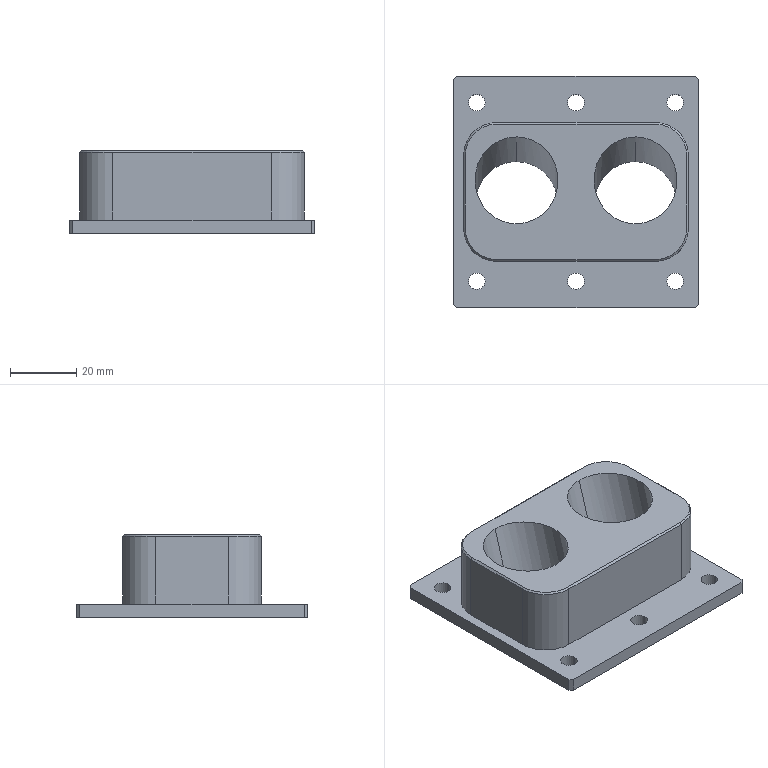Part | SolidWorks | features Chamfer 2, Extrusion 1, ICE 1, MirrorPattern 1, SweepCut 1 | 1 solid | 43 faces | box 74 x 70 x 25 mm | volume 52381 mm3 | cylinder 20 | plane 19 | cone 4 | commonest cylinder face diameters 5 x12 20 x4 25.2 x4
STEP:
#1=CARTESIAN_POINT('',(-18.,16.631,25.));
#2=VERTEX_POINT('',#1);
#3=CARTESIAN_POINT('',(-18.,-9.651,25.));
#4=VERTEX_POINT('',#3);
#5=CARTESIAN_POINT('',(-18.,16.631,25.));
#6=CARTESIAN_POINT('',(-43.2,16.631,25.));
#7=CARTESIAN_POINT('',(-43.2,-9.651,25.));
#8=CARTESIAN_POINT('',(-18.,-9.651,25.));
#9=(BOUNDED_CURVE()B_SPLINE_CURVE(3,(#5,#6,#7,#8),.UNSPECIFIED.,.F.,.F.)B_SPLINE_CURVE_WITH_KNOTS((4,4),(3.142,6.283),.UNSPECIFIED.)CURVE()GEOMETRIC_REPRESENTATION_ITEM()RATIONAL_B_SPLINE_CURVE((1.,0.3333,0.3333,1.))REPRESENTATION_ITEM(''));
#10=EDGE_CURVE('',#2,#4,#9,.T.);
#11=ORIENTED_EDGE('',*,*,#10,.T.);
#12=CARTESIAN_POINT('',(-18.,-17.056,0.));
#13=VERTEX_POINT('',#12);
#14=CARTESIAN_POINT('',(-18.,-7.234,33.159));
#15=DIRECTION('',(0.,-0.284,-0.9588));
#16=VECTOR('',#15,1000.);
#17=LINE('',#14,#16);
#18=EDGE_CURVE('',#4,#13,#17,.T.);
#19=ORIENTED_EDGE('',*,*,#18,.T.);
#20=CARTESIAN_POINT('',(-18.,9.226,0.));
#21=VERTEX_POINT('',#20);
#22=CARTESIAN_POINT('',(-18.,-17.056,0.));
#23=CARTESIAN_POINT('',(-43.2,-17.056,0.));
#24=CARTESIAN_POINT('',(-43.2,9.226,0.));
#25=CARTESIAN_POINT('',(-18.,9.226,0.));
#26=(BOUNDED_CURVE()B_SPLINE_CURVE(3,(#22,#23,#24,#25),.UNSPECIFIED.,.F.,.F.)B_SPLINE_CURVE_WITH_KNOTS((4,4),(0.,3.142),.UNSPECIFIED.)CURVE()GEOMETRIC_REPRESENTATION_ITEM()RATIONAL_B_SPLINE_CURVE((1.,0.3333,0.3333,1.))REPRESENTATION_ITEM(''));
#27=EDGE_CURVE('',#13,#21,#26,.T.);
#28=ORIENTED_EDGE('',*,*,#27,.T.);
#29=CARTESIAN_POINT('',(-18.,16.928,26.002));
#30=DIRECTION('',(0.,-0.284,-0.9588));
#31=VECTOR('',#30,1000.);
#32=LINE('',#29,#31);
#33=EDGE_CURVE('',#2,#21,#32,.T.);
#34=ORIENTED_EDGE('',*,*,#33,.F.);
#35=EDGE_LOOP('',(#11,#19,#28,#34));
#36=FACE_OUTER_BOUND('',#35,.T.);
#37=CARTESIAN_POINT('',(-18.,4.847,29.581));
#38=DIRECTION('',(0.,-0.284,-0.9588));
#39=DIRECTION('',(0.,0.9588,-0.284));
#40=AXIS2_PLACEMENT_3D('',#37,#38,#39);
#41=CYLINDRICAL_SURFACE('',#40,12.6);
#42=ADVANCED_FACE('',(#36),#41,.F.);
#43=CARTESIAN_POINT('',(18.,16.631,25.));
#44=VERTEX_POINT('',#43);
#45=CARTESIAN_POINT('',(18.,-9.651,25.));
#46=VERTEX_POINT('',#45);
#47=CARTESIAN_POINT('',(18.,16.631,25.));
#48=CARTESIAN_POINT('',(-7.2,16.631,25.));
#49=CARTESIAN_POINT('',(-7.2,-9.651,25.));
#50=CARTESIAN_POINT('',(18.,-9.651,25.));
#51=(BOUNDED_CURVE()B_SPLINE_CURVE(3,(#47,#48,#49,#50),.UNSPECIFIED.,.F.,.F.)B_SPLINE_CURVE_WITH_KNOTS((4,4),(3.142,6.283),.UNSPECIFIED.)CURVE()GEOMETRIC_REPRESENTATION_ITEM()RATIONAL_B_SPLINE_CURVE((1.,0.3333,0.3333,1.))REPRESENTATION_ITEM(''));
#52=EDGE_CURVE('',#44,#46,#51,.T.);
#53=ORIENTED_EDGE('',*,*,#52,.T.);
#54=CARTESIAN_POINT('',(18.,-17.056,0.));
#55=VERTEX_POINT('',#54);
#56=CARTESIAN_POINT('',(18.,-7.234,33.159));
#57=DIRECTION('',(0.,-0.284,-0.9588));
#58=VECTOR('',#57,1000.);
#59=LINE('',#56,#58);
#60=EDGE_CURVE('',#46,#55,#59,.T.);
#61=ORIENTED_EDGE('',*,*,#60,.T.);
#62=CARTESIAN_POINT('',(18.,9.226,0.));
#63=VERTEX_POINT('',#62);
#64=CARTESIAN_POINT('',(18.,-17.056,0.));
#65=CARTESIAN_POINT('',(-7.2,-17.056,0.));
#66=CARTESIAN_POINT('',(-7.2,9.226,0.));
#67=CARTESIAN_POINT('',(18.,9.226,0.));
#68=(BOUNDED_CURVE()B_SPLINE_CURVE(3,(#64,#65,#66,#67),.UNSPECIFIED.,.F.,.F.)B_SPLINE_CURVE_WITH_KNOTS((4,4),(0.,3.142),.UNSPECIFIED.)CURVE()GEOMETRIC_REPRESENTATION_ITEM()RATIONAL_B_SPLINE_CURVE((1.,0.3333,0.3333,1.))REPRESENTATION_ITEM(''));
#69=EDGE_CURVE('',#55,#63,#68,.T.);
#70=ORIENTED_EDGE('',*,*,#69,.T.);
#71=CARTESIAN_POINT('',(18.,16.928,26.002));
#72=DIRECTION('',(0.,-0.284,-0.9588));
#73=VECTOR('',#72,1000.);
#74=LINE('',#71,#73);
#75=EDGE_CURVE('',#44,#63,#74,.T.);
#76=ORIENTED_EDGE('',*,*,#75,.F.);
#77=EDGE_LOOP('',(#53,#61,#70,#76));
#78=FACE_OUTER_BOUND('',#77,.T.);
#79=CARTESIAN_POINT('',(18.,4.847,29.581));
#80=DIRECTION('',(0.,-0.284,-0.9588));
#81=DIRECTION('',(0.,0.9588,-0.284));
#82=AXIS2_PLACEMENT_3D('',#79,#80,#81);
#83=CYLINDRICAL_SURFACE('',#82,12.6);
#84=ADVANCED_FACE('',(#78),#83,.F.);
#85=CARTESIAN_POINT('',(-32.5,-27.,4.));
#86=VERTEX_POINT('',#85);
#87=CARTESIAN_POINT('',(-27.5,-27.,4.));
#88=VERTEX_POINT('',#87);
#89=CARTESIAN_POINT('',(-30.,-27.,4.));
#90=DIRECTION('',(0.,0.,1.));
#91=DIRECTION('',(1.,0.,0.));
#92=AXIS2_PLACEMENT_3D('',#89,#90,#91);
#93=CIRCLE('',#92,2.5);
#94=EDGE_CURVE('',#86,#88,#93,.T.);
#95=ORIENTED_EDGE('',*,*,#94,.T.);
#96=CARTESIAN_POINT('',(-27.5,-27.,0.));
#97=VERTEX_POINT('',#96);
#98=CARTESIAN_POINT('',(-27.5,-27.,4.));
#99=DIRECTION('',(0.,0.,-1.));
#100=VECTOR('',#99,1000.);
#101=LINE('',#98,#100);
#102=EDGE_CURVE('',#88,#97,#101,.T.);
#103=ORIENTED_EDGE('',*,*,#102,.T.);
#104=CARTESIAN_POINT('',(-32.5,-27.,0.));
#105=VERTEX_POINT('',#104);
#106=CARTESIAN_POINT('',(-30.,-27.,0.));
#107=DIRECTION('',(0.,0.,1.));
#108=DIRECTION('',(1.,0.,0.));
#109=AXIS2_PLACEMENT_3D('',#106,#107,#108);
#110=CIRCLE('',#109,2.5);
#111=EDGE_CURVE('',#105,#97,#110,.T.);
#112=ORIENTED_EDGE('',*,*,#111,.F.);
#113=CARTESIAN_POINT('',(-32.5,-27.,4.));
#114=DIRECTION('',(0.,0.,-1.));
#115=VECTOR('',#114,1000.);
#116=LINE('',#113,#115);
#117=EDGE_CURVE('',#86,#105,#116,.T.);
#118=ORIENTED_EDGE('',*,*,#117,.F.);
#119=EDGE_LOOP('',(#95,#103,#112,#118));
#120=FACE_OUTER_BOUND('',#119,.T.);
#121=CARTESIAN_POINT('',(-30.,-27.,4.));
#122=DIRECTION('',(0.,0.,-1.));
#123=DIRECTION('',(-1.,0.,0.));
#124=AXIS2_PLACEMENT_3D('',#121,#122,#123);
#125=CYLINDRICAL_SURFACE('',#124,2.5);
#126=ADVANCED_FACE('',(#120),#125,.F.);
#127=CARTESIAN_POINT('',(-2.5,-27.,4.));
#128=VERTEX_POINT('',#127);
#129=CARTESIAN_POINT('',(2.5,-27.,4.));
#130=VERTEX_POINT('',#129);
#131=CARTESIAN_POINT('',(0.,-27.,4.));
#132=DIRECTION('',(0.,0.,1.));
#133=DIRECTION('',(1.,0.,0.));
#134=AXIS2_PLACEMENT_3D('',#131,#132,#133);
#135=CIRCLE('',#134,2.5);
#136=EDGE_CURVE('',#128,#130,#135,.T.);
#137=ORIENTED_EDGE('',*,*,#136,.T.);
#138=CARTESIAN_POINT('',(2.5,-27.,0.));
#139=VERTEX_POINT('',#138);
#140=CARTESIAN_POINT('',(2.5,-27.,4.));
#141=DIRECTION('',(0.,0.,-1.));
#142=VECTOR('',#141,1000.);
#143=LINE('',#140,#142);
#144=EDGE_CURVE('',#130,#139,#143,.T.);
#145=ORIENTED_EDGE('',*,*,#144,.T.);
#146=CARTESIAN_POINT('',(-2.5,-27.,0.));
#147=VERTEX_POINT('',#146);
#148=CARTESIAN_POINT('',(0.,-27.,0.));
#149=DIRECTION('',(0.,0.,1.));
#150=DIRECTION('',(1.,0.,0.));
#151=AXIS2_PLACEMENT_3D('',#148,#149,#150);
#152=CIRCLE('',#151,2.5);
#153=EDGE_CURVE('',#147,#139,#152,.T.);
#154=ORIENTED_EDGE('',*,*,#153,.F.);
#155=CARTESIAN_POINT('',(-2.5,-27.,4.));
#156=DIRECTION('',(0.,0.,-1.));
#157=VECTOR('',#156,1000.);
#158=LINE('',#155,#157);
#159=EDGE_CURVE('',#128,#147,#158,.T.);
#160=ORIENTED_EDGE('',*,*,#159,.F.);
#161=EDGE_LOOP('',(#137,#145,#154,#160));
#162=FACE_OUTER_BOUND('',#161,.T.);
#163=CARTESIAN_POINT('',(0.,-27.,4.));
#164=DIRECTION('',(0.,0.,-1.));
#165=DIRECTION('',(-1.,0.,0.));
#166=AXIS2_PLACEMENT_3D('',#163,#164,#165);
#167=CYLINDRICAL_SURFACE('',#166,2.5);
#168=ADVANCED_FACE('',(#162),#167,.F.);
#169=CARTESIAN_POINT('',(27.5,-27.,4.));
#170=VERTEX_POINT('',#169);
#171=CARTESIAN_POINT('',(32.5,-27.,4.));
#172=VERTEX_POINT('',#171);
#173=CARTESIAN_POINT('',(30.,-27.,4.));
#174=DIRECTION('',(0.,0.,1.));
#175=DIRECTION('',(1.,0.,0.));
#176=AXIS2_PLACEMENT_3D('',#173,#174,#175);
#177=CIRCLE('',#176,2.5);
#178=EDGE_CURVE('',#170,#172,#177,.T.);
#179=ORIENTED_EDGE('',*,*,#178,.T.);
#180=CARTESIAN_POINT('',(32.5,-27.,0.));
#181=VERTEX_POINT('',#180);
#182=CARTESIAN_POINT('',(32.5,-27.,4.));
#183=DIRECTION('',(0.,0.,-1.));
#184=VECTOR('',#183,1000.);
#185=LINE('',#182,#184);
#186=EDGE_CURVE('',#172,#181,#185,.T.);
#187=ORIENTED_EDGE('',*,*,#186,.T.);
#188=CARTESIAN_POINT('',(27.5,-27.,0.));
#189=VERTEX_POINT('',#188);
#190=CARTESIAN_POINT('',(30.,-27.,0.));
#191=DIRECTION('',(0.,0.,1.));
#192=DIRECTION('',(1.,0.,0.));
#193=AXIS2_PLACEMENT_3D('',#190,#191,#192);
#194=CIRCLE('',#193,2.5);
#195=EDGE_CURVE('',#189,#181,#194,.T.);
#196=ORIENTED_EDGE('',*,*,#195,.F.);
#197=CARTESIAN_POINT('',(27.5,-27.,4.));
#198=DIRECTION('',(0.,0.,-1.));
#199=VECTOR('',#198,1000.);
#200=LINE('',#197,#199);
#201=EDGE_CURVE('',#170,#189,#200,.T.);
#202=ORIENTED_EDGE('',*,*,#201,.F.);
#203=EDGE_LOOP('',(#179,#187,#196,#202));
#204=FACE_OUTER_BOUND('',#203,.T.);
#205=CARTESIAN_POINT('',(30.,-27.,4.));
#206=DIRECTION('',(0.,0.,-1.));
#207=DIRECTION('',(-1.,0.,0.));
#208=AXIS2_PLACEMENT_3D('',#205,#206,#207);
#209=CYLINDRICAL_SURFACE('',#208,2.5);
#210=ADVANCED_FACE('',(#204),#209,.F.);
#211=CARTESIAN_POINT('',(27.5,27.,4.));
#212=VERTEX_POINT('',#211);
#213=CARTESIAN_POINT('',(32.5,27.,4.));
#214=VERTEX_POINT('',#213);
#215=CARTESIAN_POINT('',(30.,27.,4.));
#216=DIRECTION('',(0.,0.,1.));
#217=DIRECTION('',(1.,0.,0.));
#218=AXIS2_PLACEMENT_3D('',#215,#216,#217);
#219=CIRCLE('',#218,2.5);
#220=EDGE_CURVE('',#212,#214,#219,.T.);
#221=ORIENTED_EDGE('',*,*,#220,.T.);
#222=CARTESIAN_POINT('',(32.5,27.,0.));
#223=VERTEX_POINT('',#222);
#224=CARTESIAN_POINT('',(32.5,27.,4.));
#225=DIRECTION('',(0.,0.,-1.));
#226=VECTOR('',#225,1000.);
#227=LINE('',#224,#226);
#228=EDGE_CURVE('',#214,#223,#227,.T.);
#229=ORIENTED_EDGE('',*,*,#228,.T.);
#230=CARTESIAN_POINT('',(27.5,27.,0.));
#231=VERTEX_POINT('',#230);
#232=CARTESIAN_POINT('',(30.,27.,0.));
#233=DIRECTION('',(0.,0.,1.));
#234=DIRECTION('',(1.,0.,0.));
#235=AXIS2_PLACEMENT_3D('',#232,#233,#234);
#236=CIRCLE('',#235,2.5);
#237=EDGE_CURVE('',#231,#223,#236,.T.);
#238=ORIENTED_EDGE('',*,*,#237,.F.);
#239=CARTESIAN_POINT('',(27.5,27.,4.));
#240=DIRECTION('',(0.,0.,-1.));
#241=VECTOR('',#240,1000.);
#242=LINE('',#239,#241);
#243=EDGE_CURVE('',#212,#231,#242,.T.);
#244=ORIENTED_EDGE('',*,*,#243,.F.);
#245=EDGE_LOOP('',(#221,#229,#238,#244));
#246=FACE_OUTER_BOUND('',#245,.T.);
#247=CARTESIAN_POINT('',(30.,27.,4.));
#248=DIRECTION('',(0.,0.,-1.));
#249=DIRECTION('',(-1.,0.,0.));
#250=AXIS2_PLACEMENT_3D('',#247,#248,#249);
#251=CYLINDRICAL_SURFACE('',#250,2.5);
#252=ADVANCED_FACE('',(#246),#251,.F.);
#253=CARTESIAN_POINT('',(-2.5,27.,4.));
#254=VERTEX_POINT('',#253);
#255=CARTESIAN_POINT('',(2.5,27.,4.));
#256=VERTEX_POINT('',#255);
#257=CARTESIAN_POINT('',(0.,27.,4.));
#258=DIRECTION('',(0.,0.,1.));
#259=DIRECTION('',(1.,0.,0.));
#260=AXIS2_PLACEMENT_3D('',#257,#258,#259);
#261=CIRCLE('',#260,2.5);
#262=EDGE_CURVE('',#254,#256,#261,.T.);
#263=ORIENTED_EDGE('',*,*,#262,.T.);
#264=CARTESIAN_POINT('',(2.5,27.,0.));
#265=VERTEX_POINT('',#264);
#266=CARTESIAN_POINT('',(2.5,27.,4.));
#267=DIRECTION('',(0.,0.,-1.));
#268=VECTOR('',#267,1000.);
#269=LINE('',#266,#268);
#270=EDGE_CURVE('',#256,#265,#269,.T.);
#271=ORIENTED_EDGE('',*,*,#270,.T.);
#272=CARTESIAN_POINT('',(-2.5,27.,0.));
#273=VERTEX_POINT('',#272);
#274=CARTESIAN_POINT('',(0.,27.,0.));
#275=DIRECTION('',(0.,0.,1.));
#276=DIRECTION('',(1.,0.,0.));
#277=AXIS2_PLACEMENT_3D('',#274,#275,#276);
#278=CIRCLE('',#277,2.5);
#279=EDGE_CURVE('',#273,#265,#278,.T.);
#280=ORIENTED_EDGE('',*,*,#279,.F.);
#281=CARTESIAN_POINT('',(-2.5,27.,4.));
#282=DIRECTION('',(0.,0.,-1.));
#283=VECTOR('',#282,1000.);
#284=LINE('',#281,#283);
#285=EDGE_CURVE('',#254,#273,#284,.T.);
#286=ORIENTED_EDGE('',*,*,#285,.F.);
#287=EDGE_LOOP('',(#263,#271,#280,#286));
#288=FACE_OUTER_BOUND('',#287,.T.);
#289=CARTESIAN_POINT('',(0.,27.,4.));
#290=DIRECTION('',(0.,0.,-1.));
#291=DIRECTION('',(-1.,0.,0.));
#292=AXIS2_PLACEMENT_3D('',#289,#290,#291);
#293=CYLINDRICAL_SURFACE('',#292,2.5);
#294=ADVANCED_FACE('',(#288),#293,.F.);
#295=CARTESIAN_POINT('',(-32.5,27.,4.));
#296=VERTEX_POINT('',#295);
#297=CARTESIAN_POINT('',(-27.5,27.,4.));
#298=VERTEX_POINT('',#297);
#299=CARTESIAN_POINT('',(-30.,27.,4.));
#300=DIRECTION('',(0.,0.,1.));
#301=DIRECTION('',(1.,0.,0.));
#302=AXIS2_PLACEMENT_3D('',#299,#300,#301);
#303=CIRCLE('',#302,2.5);
#304=EDGE_CURVE('',#296,#298,#303,.T.);
#305=ORIENTED_EDGE('',*,*,#304,.T.);
#306=CARTESIAN_POINT('',(-27.5,27.,0.));
#307=VERTEX_POINT('',#306);
#308=CARTESIAN_POINT('',(-27.5,27.,4.));
#309=DIRECTION('',(0.,0.,-1.));
#310=VECTOR('',#309,1000.);
#311=LINE('',#308,#310);
#312=EDGE_CURVE('',#298,#307,#311,.T.);
#313=ORIENTED_EDGE('',*,*,#312,.T.);
#314=CARTESIAN_POINT('',(-32.5,27.,0.));
#315=VERTEX_POINT('',#314);
#316=CARTESIAN_POINT('',(-30.,27.,0.));
#317=DIRECTION('',(0.,0.,1.));
#318=DIRECTION('',(1.,0.,0.));
#319=AXIS2_PLACEMENT_3D('',#316,#317,#318);
#320=CIRCLE('',#319,2.5);
#321=EDGE_CURVE('',#315,#307,#320,.T.);
#322=ORIENTED_EDGE('',*,*,#321,.F.);
#323=CARTESIAN_POINT('',(-32.5,27.,4.));
#324=DIRECTION('',(0.,0.,-1.));
#325=VECTOR('',#324,1000.);
#326=LINE('',#323,#325);
#327=EDGE_CURVE('',#296,#315,#326,.T.);
#328=ORIENTED_EDGE('',*,*,#327,.F.);
#329=EDGE_LOOP('',(#305,#313,#322,#328));
#330=FACE_OUTER_BOUND('',#329,.T.);
#331=CARTESIAN_POINT('',(-30.,27.,4.));
#332=DIRECTION('',(0.,0.,-1.));
#333=DIRECTION('',(-1.,0.,0.));
#334=AXIS2_PLACEMENT_3D('',#331,#332,#333);
#335=CYLINDRICAL_SURFACE('',#334,2.5);
#336=ADVANCED_FACE('',(#330),#335,.F.);
#337=ORIENTED_EDGE('',*,*,#94,.F.);
#338=CARTESIAN_POINT('',(-30.,-27.,4.));
#339=DIRECTION('',(0.,0.,1.));
#340=DIRECTION('',(1.,0.,0.));
#341=AXIS2_PLACEMENT_3D('',#338,#339,#340);
#342=CIRCLE('',#341,2.5);
#343=EDGE_CURVE('',#88,#86,#342,.T.);
#344=ORIENTED_EDGE('',*,*,#343,.F.);
#345=EDGE_LOOP('',(#337,#344));
#346=FACE_BOUND('',#345,.T.);
#347=ORIENTED_EDGE('',*,*,#136,.F.);
#348=CARTESIAN_POINT('',(0.,-27.,4.));
#349=DIRECTION('',(0.,0.,1.));
#350=DIRECTION('',(1.,0.,0.));
#351=AXIS2_PLACEMENT_3D('',#348,#349,#350);
#352=CIRCLE('',#351,2.5);
#353=EDGE_CURVE('',#130,#128,#352,.T.);
#354=ORIENTED_EDGE('',*,*,#353,.F.);
#355=EDGE_LOOP('',(#347,#354));
#356=FACE_BOUND('',#355,.T.);
#357=ORIENTED_EDGE('',*,*,#178,.F.);
#358=CARTESIAN_POINT('',(30.,-27.,4.));
#359=DIRECTION('',(0.,0.,1.));
#360=DIRECTION('',(1.,0.,0.));
#361=AXIS2_PLACEMENT_3D('',#358,#359,#360);
#362=CIRCLE('',#361,2.5);
#363=EDGE_CURVE('',#172,#170,#362,.T.);
#364=ORIENTED_EDGE('',*,*,#363,.F.);
#365=EDGE_LOOP('',(#357,#364));
#366=FACE_BOUND('',#365,.T.);
#367=ORIENTED_EDGE('',*,*,#220,.F.);
#368=CARTESIAN_POINT('',(30.,27.,4.));
#369=DIRECTION('',(0.,0.,1.));
#370=DIRECTION('',(1.,0.,0.));
#371=AXIS2_PLACEMENT_3D('',#368,#369,#370);
#372=CIRCLE('',#371,2.5);
#373=EDGE_CURVE('',#214,#212,#372,.T.);
#374=ORIENTED_EDGE('',*,*,#373,.F.);
#375=EDGE_LOOP('',(#367,#374));
#376=FACE_BOUND('',#375,.T.);
#377=ORIENTED_EDGE('',*,*,#262,.F.);
#378=CARTESIAN_POINT('',(0.,27.,4.));
#379=DIRECTION('',(0.,0.,1.));
#380=DIRECTION('',(1.,0.,0.));
#381=AXIS2_PLACEMENT_3D('',#378,#379,#380);
#382=CIRCLE('',#381,2.5);
#383=EDGE_CURVE('',#256,#254,#382,.T.);
#384=ORIENTED_EDGE('',*,*,#383,.F.);
#385=EDGE_LOOP('',(#377,#384));
#386=FACE_BOUND('',#385,.T.);
#387=ORIENTED_EDGE('',*,*,#304,.F.);
#388=CARTESIAN_POINT('',(-30.,27.,4.));
#389=DIRECTION('',(0.,0.,1.));
#390=DIRECTION('',(1.,0.,0.));
#391=AXIS2_PLACEMENT_3D('',#388,#389,#390);
#392=CIRCLE('',#391,2.5);
#393=EDGE_CURVE('',#298,#296,#392,.T.);
#394=ORIENTED_EDGE('',*,*,#393,.F.);
#395=EDGE_LOOP('',(#387,#394));
#396=FACE_BOUND('',#395,.T.);
#397=CARTESIAN_POINT('',(-36.,-35.,4.));
#398=VERTEX_POINT('',#397);
#399=CARTESIAN_POINT('',(36.,-35.,4.));
#400=VERTEX_POINT('',#399);
#401=CARTESIAN_POINT('',(0.,-35.,4.));
#402=DIRECTION('',(1.,0.,0.));
#403=VECTOR('',#402,1000.);
#404=LINE('',#401,#403);
#405=EDGE_CURVE('',#398,#400,#404,.T.);
#406=ORIENTED_EDGE('',*,*,#405,.T.);
#407=CARTESIAN_POINT('',(37.,-34.,4.));
#408=VERTEX_POINT('',#407);
#409=CARTESIAN_POINT('',(35.5,-35.5,4.));
#410=DIRECTION('',(0.7071,0.7071,0.));
#411=VECTOR('',#410,1000.);
#412=LINE('',#409,#411);
#413=EDGE_CURVE('',#400,#408,#412,.T.);
#414=ORIENTED_EDGE('',*,*,#413,.T.);
#415=CARTESIAN_POINT('',(37.,34.,4.));
#416=VERTEX_POINT('',#415);
#417=CARTESIAN_POINT('',(37.,0.,4.));
#418=DIRECTION('',(0.,1.,0.));
#419=VECTOR('',#418,1000.);
#420=LINE('',#417,#419);
#421=EDGE_CURVE('',#408,#416,#420,.T.);
#422=ORIENTED_EDGE('',*,*,#421,.T.);
#423=CARTESIAN_POINT('',(36.,35.,4.));
#424=VERTEX_POINT('',#423);
#425=CARTESIAN_POINT('',(35.5,35.5,4.));
#426=DIRECTION('',(-0.7071,0.7071,0.));
#427=VECTOR('',#426,1000.);
#428=LINE('',#425,#427);
#429=EDGE_CURVE('',#416,#424,#428,.T.);
#430=ORIENTED_EDGE('',*,*,#429,.T.);
#431=CARTESIAN_POINT('',(-36.,35.,4.));
#432=VERTEX_POINT('',#431);
#433=CARTESIAN_POINT('',(0.,35.,4.));
#434=DIRECTION('',(1.,0.,0.));
#435=VECTOR('',#434,1000.);
#436=LINE('',#433,#435);
#437=EDGE_CURVE('',#432,#424,#436,.T.);
#438=ORIENTED_EDGE('',*,*,#437,.F.);
#439=CARTESIAN_POINT('',(-37.,34.,4.));
#440=VERTEX_POINT('',#439);
#441=CARTESIAN_POINT('',(-35.5,35.5,4.));
#442=DIRECTION('',(-0.7071,-0.7071,0.));
#443=VECTOR('',#442,1000.);
#444=LINE('',#441,#443);
#445=EDGE_CURVE('',#432,#440,#444,.T.);
#446=ORIENTED_EDGE('',*,*,#445,.T.);
#447=CARTESIAN_POINT('',(-37.,-34.,4.));
#448=VERTEX_POINT('',#447);
#449=CARTESIAN_POINT('',(-37.,0.,4.));
#450=DIRECTION('',(0.,1.,0.));
#451=VECTOR('',#450,1000.);
#452=LINE('',#449,#451);
#453=EDGE_CURVE('',#448,#440,#452,.T.);
#454=ORIENTED_EDGE('',*,*,#453,.F.);
#455=CARTESIAN_POINT('',(-35.5,-35.5,4.));
#456=DIRECTION('',(0.7071,-0.7071,0.));
#457=VECTOR('',#456,1000.);
#458=LINE('',#455,#457);
#459=EDGE_CURVE('',#448,#398,#458,.T.);
#460=ORIENTED_EDGE('',*,*,#459,.T.);
#461=EDGE_LOOP('',(#406,#414,#422,#430,#438,#446,#454,#460));
#462=FACE_OUTER_BOUND('',#461,.T.);
#463=CARTESIAN_POINT('',(24.,21.,4.));
#464=VERTEX_POINT('',#463);
#465=CARTESIAN_POINT('',(-24.,21.,4.));
#466=VERTEX_POINT('',#465);
#467=CARTESIAN_POINT('',(-24.,21.,4.));
#468=DIRECTION('',(-1.,0.,0.));
#469=VECTOR('',#468,1000.);
#470=LINE('',#467,#469);
#471=EDGE_CURVE('',#464,#466,#470,.T.);
#472=ORIENTED_EDGE('',*,*,#471,.F.);
#473=CARTESIAN_POINT('',(34.,11.,4.));
#474=VERTEX_POINT('',#473);
#475=CARTESIAN_POINT('',(24.,11.,4.));
#476=DIRECTION('',(0.,0.,1.));
#477=DIRECTION('',(-1.,0.,0.));
#478=AXIS2_PLACEMENT_3D('',#475,#476,#477);
#479=CIRCLE('',#478,10.);
#480=EDGE_CURVE('',#474,#464,#479,.T.);
#481=ORIENTED_EDGE('',*,*,#480,.F.);
#482=CARTESIAN_POINT('',(34.,-11.,4.));
#483=VERTEX_POINT('',#482);
#484=CARTESIAN_POINT('',(34.,-11.,4.));
#485=DIRECTION('',(0.,1.,0.));
#486=VECTOR('',#485,1000.);
#487=LINE('',#484,#486);
#488=EDGE_CURVE('',#483,#474,#487,.T.);
#489=ORIENTED_EDGE('',*,*,#488,.F.);
#490=CARTESIAN_POINT('',(24.,-21.,4.));
#491=VERTEX_POINT('',#490);
#492=CARTESIAN_POINT('',(24.,-11.,4.));
#493=DIRECTION('',(0.,0.,1.));
#494=DIRECTION('',(-1.,0.,0.));
#495=AXIS2_PLACEMENT_3D('',#492,#493,#494);
#496=CIRCLE('',#495,10.);
#497=EDGE_CURVE('',#491,#483,#496,.T.);
#498=ORIENTED_EDGE('',*,*,#497,.F.);
#499=CARTESIAN_POINT('',(-24.,-21.,4.));
#500=VERTEX_POINT('',#499);
#501=CARTESIAN_POINT('',(-24.,-21.,4.));
#502=DIRECTION('',(1.,0.,0.));
#503=VECTOR('',#502,1000.);
#504=LINE('',#501,#503);
#505=EDGE_CURVE('',#500,#491,#504,.T.);
#506=ORIENTED_EDGE('',*,*,#505,.F.);
#507=CARTESIAN_POINT('',(-34.,-11.,4.));
#508=VERTEX_POINT('',#507);
#509=CARTESIAN_POINT('',(-24.,-11.,4.));
#510=DIRECTION('',(0.,0.,1.));
#511=DIRECTION('',(-1.,0.,0.));
#512=AXIS2_PLACEMENT_3D('',#509,#510,#511);
#513=CIRCLE('',#512,10.);
#514=EDGE_CURVE('',#508,#500,#513,.T.);
#515=ORIENTED_EDGE('',*,*,#514,.F.);
#516=CARTESIAN_POINT('',(-34.,11.,4.));
#517=VERTEX_POINT('',#516);
#518=CARTESIAN_POINT('',(-34.,-11.,4.));
#519=DIRECTION('',(0.,-1.,0.));
#520=VECTOR('',#519,1000.);
#521=LINE('',#518,#520);
#522=EDGE_CURVE('',#517,#508,#521,.T.);
#523=ORIENTED_EDGE('',*,*,#522,.F.);
#524=CARTESIAN_POINT('',(-24.,11.,4.));
#525=DIRECTION('',(0.,0.,1.));
#526=DIRECTION('',(-1.,0.,0.));
#527=AXIS2_PLACEMENT_3D('',#524,#525,#526);
#528=CIRCLE('',#527,10.);
#529=EDGE_CURVE('',#466,#517,#528,.T.);
#530=ORIENTED_EDGE('',*,*,#529,.F.);
#531=EDGE_LOOP('',(#472,#481,#489,#498,#506,#515,#523,#530));
#532=FACE_BOUND('',#531,.T.);
#533=CARTESIAN_POINT('',(0.,0.,4.));
#534=DIRECTION('',(0.,0.,1.));
#535=DIRECTION('',(1.,0.,0.));
#536=AXIS2_PLACEMENT_3D('',#533,#534,#535);
#537=PLANE('',#536);
#538=ADVANCED_FACE('',(#346,#356,#366,#376,#386,#396,#462,#532),#537,.T.);
#539=CARTESIAN_POINT('',(-36.,-35.,0.));
#540=VERTEX_POINT('',#539);
#541=CARTESIAN_POINT('',(36.,-35.,0.));
#542=VERTEX_POINT('',#541);
#543=CARTESIAN_POINT('',(0.,-35.,0.));
#544=DIRECTION('',(1.,0.,0.));
#545=VECTOR('',#544,1000.);
#546=LINE('',#543,#545);
#547=EDGE_CURVE('',#540,#542,#546,.T.);
#548=ORIENTED_EDGE('',*,*,#547,.T.);
#549=CARTESIAN_POINT('',(36.,-35.,4.));
#550=DIRECTION('',(0.,0.,1.));
#551=VECTOR('',#550,1000.);
#552=LINE('',#549,#551);
#553=EDGE_CURVE('',#542,#400,#552,.T.);
#554=ORIENTED_EDGE('',*,*,#553,.T.);
#555=ORIENTED_EDGE('',*,*,#405,.F.);
#556=CARTESIAN_POINT('',(-36.,-35.,0.));
#557=DIRECTION('',(0.,0.,-1.));
#558=VECTOR('',#557,1000.);
#559=LINE('',#556,#558);
#560=EDGE_CURVE('',#398,#540,#559,.T.);
#561=ORIENTED_EDGE('',*,*,#560,.T.);
#562=EDGE_LOOP('',(#548,#554,#555,#561));
#563=FACE_OUTER_BOUND('',#562,.T.);
#564=CARTESIAN_POINT('',(0.,-35.,4.));
#565=DIRECTION('',(0.,1.,0.));
#566=DIRECTION('',(0.,0.,1.));
#567=AXIS2_PLACEMENT_3D('',#564,#565,#566);
#568=PLANE('',#567);
#569=ADVANCED_FACE('',(#563),#568,.F.);
#570=ORIENTED_EDGE('',*,*,#421,.F.);
#571=CARTESIAN_POINT('',(37.,-34.,0.));
#572=VERTEX_POINT('',#571);
#573=CARTESIAN_POINT('',(37.,-34.,4.));
#574=DIRECTION('',(0.,0.,-1.));
#575=VECTOR('',#574,1000.);
#576=LINE('',#573,#575);
#577=EDGE_CURVE('',#408,#572,#576,.T.);
#578=ORIENTED_EDGE('',*,*,#577,.T.);
#579=CARTESIAN_POINT('',(37.,34.,0.));
#580=VERTEX_POINT('',#579);
#581=CARTESIAN_POINT('',(37.,0.,0.));
#582=DIRECTION('',(0.,1.,0.));
#583=VECTOR('',#582,1000.);
#584=LINE('',#581,#583);
#585=EDGE_CURVE('',#572,#580,#584,.T.);
#586=ORIENTED_EDGE('',*,*,#585,.T.);
#587=CARTESIAN_POINT('',(37.,34.,4.));
#588=DIRECTION('',(0.,0.,1.));
#589=VECTOR('',#588,1000.);
#590=LINE('',#587,#589);
#591=EDGE_CURVE('',#580,#416,#590,.T.);
#592=ORIENTED_EDGE('',*,*,#591,.T.);
#593=EDGE_LOOP('',(#570,#578,#586,#592));
#594=FACE_OUTER_BOUND('',#593,.T.);
#595=CARTESIAN_POINT('',(37.,0.,4.));
#596=DIRECTION('',(-1.,0.,0.));
#597=DIRECTION('',(0.,0.,1.));
#598=AXIS2_PLACEMENT_3D('',#595,#596,#597);
#599=PLANE('',#598);
#600=ADVANCED_FACE('',(#594),#599,.F.);
#601=ORIENTED_EDGE('',*,*,#437,.T.);
#602=CARTESIAN_POINT('',(36.,35.,0.));
#603=VERTEX_POINT('',#602);
#604=CARTESIAN_POINT('',(36.,35.,0.));
#605=DIRECTION('',(0.,0.,-1.));
#606=VECTOR('',#605,1000.);
#607=LINE('',#604,#606);
#608=EDGE_CURVE('',#424,#603,#607,.T.);
#609=ORIENTED_EDGE('',*,*,#608,.T.);
#610=CARTESIAN_POINT('',(-36.,35.,0.));
#611=VERTEX_POINT('',#610);
#612=CARTESIAN_POINT('',(0.,35.,0.));
#613=DIRECTION('',(1.,0.,0.));
#614=VECTOR('',#613,1000.);
#615=LINE('',#612,#614);
#616=EDGE_CURVE('',#611,#603,#615,.T.);
#617=ORIENTED_EDGE('',*,*,#616,.F.);
#618=CARTESIAN_POINT('',(-36.,35.,4.));
#619=DIRECTION('',(0.,0.,1.));
#620=VECTOR('',#619,1000.);
#621=LINE('',#618,#620);
#622=EDGE_CURVE('',#611,#432,#621,.T.);
#623=ORIENTED_EDGE('',*,*,#622,.T.);
#624=EDGE_LOOP('',(#601,#609,#617,#623));
#625=FACE_OUTER_BOUND('',#624,.T.);
#626=CARTESIAN_POINT('',(0.,35.,4.));
#627=DIRECTION('',(0.,1.,0.));
#628=DIRECTION('',(0.,0.,1.));
#629=AXIS2_PLACEMENT_3D('',#626,#627,#628);
#630=PLANE('',#629);
#631=ADVANCED_FACE('',(#625),#630,.T.);
#632=ORIENTED_EDGE('',*,*,#312,.F.);
#633=ORIENTED_EDGE('',*,*,#393,.T.);
#634=ORIENTED_EDGE('',*,*,#327,.T.);
#635=CARTESIAN_POINT('',(-30.,27.,0.));
#636=DIRECTION('',(0.,0.,1.));
#637=DIRECTION('',(1.,0.,0.));
#638=AXIS2_PLACEMENT_3D('',#635,#636,#637);
#639=CIRCLE('',#638,2.5);
#640=EDGE_CURVE('',#307,#315,#639,.T.);
#641=ORIENTED_EDGE('',*,*,#640,.F.);
#642=EDGE_LOOP('',(#632,#633,#634,#641));
#643=FACE_OUTER_BOUND('',#642,.T.);
#644=CARTESIAN_POINT('',(-30.,27.,4.));
#645=DIRECTION('',(0.,0.,-1.));
#646=DIRECTION('',(-1.,0.,0.));
#647=AXIS2_PLACEMENT_3D('',#644,#645,#646);
#648=CYLINDRICAL_SURFACE('',#647,2.5);
#649=ADVANCED_FACE('',(#643),#648,.F.);
#650=ORIENTED_EDGE('',*,*,#270,.F.);
#651=ORIENTED_EDGE('',*,*,#383,.T.);
#652=ORIENTED_EDGE('',*,*,#285,.T.);
#653=CARTESIAN_POINT('',(0.,27.,0.));
#654=DIRECTION('',(0.,0.,1.));
#655=DIRECTION('',(1.,0.,0.));
#656=AXIS2_PLACEMENT_3D('',#653,#654,#655);
#657=CIRCLE('',#656,2.5);
#658=EDGE_CURVE('',#265,#273,#657,.T.);
#659=ORIENTED_EDGE('',*,*,#658,.F.);
#660=EDGE_LOOP('',(#650,#651,#652,#659));
#661=FACE_OUTER_BOUND('',#660,.T.);
#662=CARTESIAN_POINT('',(0.,27.,4.));
#663=DIRECTION('',(0.,0.,-1.));
#664=DIRECTION('',(-1.,0.,0.));
#665=AXIS2_PLACEMENT_3D('',#662,#663,#664);
#666=CYLINDRICAL_SURFACE('',#665,2.5);
#667=ADVANCED_FACE('',(#661),#666,.F.);
#668=ORIENTED_EDGE('',*,*,#228,.F.);
#669=ORIENTED_EDGE('',*,*,#373,.T.);
#670=ORIENTED_EDGE('',*,*,#243,.T.);
#671=CARTESIAN_POINT('',(30.,27.,0.));
#672=DIRECTION('',(0.,0.,1.));
#673=DIRECTION('',(1.,0.,0.));
#674=AXIS2_PLACEMENT_3D('',#671,#672,#673);
#675=CIRCLE('',#674,2.5);
#676=EDGE_CURVE('',#223,#231,#675,.T.);
#677=ORIENTED_EDGE('',*,*,#676,.F.);
#678=EDGE_LOOP('',(#668,#669,#670,#677));
#679=FACE_OUTER_BOUND('',#678,.T.);
#680=CARTESIAN_POINT('',(30.,27.,4.));
#681=DIRECTION('',(0.,0.,-1.));
#682=DIRECTION('',(-1.,0.,0.));
#683=AXIS2_PLACEMENT_3D('',#680,#681,#682);
#684=CYLINDRICAL_SURFACE('',#683,2.5);
#685=ADVANCED_FACE('',(#679),#684,.F.);
#686=ORIENTED_EDGE('',*,*,#186,.F.);
#687=ORIENTED_EDGE('',*,*,#363,.T.);
#688=ORIENTED_EDGE('',*,*,#201,.T.);
#689=CARTESIAN_POINT('',(30.,-27.,0.));
#690=DIRECTION('',(0.,0.,1.));
#691=DIRECTION('',(1.,0.,0.));
#692=AXIS2_PLACEMENT_3D('',#689,#690,#691);
#693=CIRCLE('',#692,2.5);
#694=EDGE_CURVE('',#181,#189,#693,.T.);
#695=ORIENTED_EDGE('',*,*,#694,.F.);
#696=EDGE_LOOP('',(#686,#687,#688,#695));
#697=FACE_OUTER_BOUND('',#696,.T.);
#698=CARTESIAN_POINT('',(30.,-27.,4.));
#699=DIRECTION('',(0.,0.,-1.));
#700=DIRECTION('',(-1.,0.,0.));
#701=AXIS2_PLACEMENT_3D('',#698,#699,#700);
#702=CYLINDRICAL_SURFACE('',#701,2.5);
#703=ADVANCED_FACE('',(#697),#702,.F.);
#704=ORIENTED_EDGE('',*,*,#144,.F.);
#705=ORIENTED_EDGE('',*,*,#353,.T.);
#706=ORIENTED_EDGE('',*,*,#159,.T.);
#707=CARTESIAN_POINT('',(0.,-27.,0.));
#708=DIRECTION('',(0.,0.,1.));
#709=DIRECTION('',(1.,0.,0.));
#710=AXIS2_PLACEMENT_3D('',#707,#708,#709);
#711=CIRCLE('',#710,2.5);
#712=EDGE_CURVE('',#139,#147,#711,.T.);
#713=ORIENTED_EDGE('',*,*,#712,.F.);
#714=EDGE_LOOP('',(#704,#705,#706,#713));
#715=FACE_OUTER_BOUND('',#714,.T.);
#716=CARTESIAN_POINT('',(0.,-27.,4.));
#717=DIRECTION('',(0.,0.,-1.));
#718=DIRECTION('',(-1.,0.,0.));
#719=AXIS2_PLACEMENT_3D('',#716,#717,#718);
#720=CYLINDRICAL_SURFACE('',#719,2.5);
#721=ADVANCED_FACE('',(#715),#720,.F.);
#722=ORIENTED_EDGE('',*,*,#102,.F.);
#723=ORIENTED_EDGE('',*,*,#343,.T.);
#724=ORIENTED_EDGE('',*,*,#117,.T.);
#725=CARTESIAN_POINT('',(-30.,-27.,0.));
#726=DIRECTION('',(0.,0.,1.));
#727=DIRECTION('',(1.,0.,0.));
#728=AXIS2_PLACEMENT_3D('',#725,#726,#727);
#729=CIRCLE('',#728,2.5);
#730=EDGE_CURVE('',#97,#105,#729,.T.);
#731=ORIENTED_EDGE('',*,*,#730,.F.);
#732=EDGE_LOOP('',(#722,#723,#724,#731));
#733=FACE_OUTER_BOUND('',#732,.T.);
#734=CARTESIAN_POINT('',(-30.,-27.,4.));
#735=DIRECTION('',(0.,0.,-1.));
#736=DIRECTION('',(-1.,0.,0.));
#737=AXIS2_PLACEMENT_3D('',#734,#735,#736);
#738=CYLINDRICAL_SURFACE('',#737,2.5);
#739=ADVANCED_FACE('',(#733),#738,.F.);
#740=CARTESIAN_POINT('',(-37.,-34.,0.));
#741=VERTEX_POINT('',#740);
#742=CARTESIAN_POINT('',(-37.,34.,0.));
#743=VERTEX_POINT('',#742);
#744=CARTESIAN_POINT('',(-37.,0.,0.));
#745=DIRECTION('',(0.,1.,0.));
#746=VECTOR('',#745,1000.);
#747=LINE('',#744,#746);
#748=EDGE_CURVE('',#741,#743,#747,.T.);
#749=ORIENTED_EDGE('',*,*,#748,.F.);
#750=CARTESIAN_POINT('',(-37.,-34.,4.));
#751=DIRECTION('',(0.,0.,1.));
#752=VECTOR('',#751,1000.);
#753=LINE('',#750,#752);
#754=EDGE_CURVE('',#741,#448,#753,.T.);
#755=ORIENTED_EDGE('',*,*,#754,.T.);
#756=ORIENTED_EDGE('',*,*,#453,.T.);
#757=CARTESIAN_POINT('',(-37.,34.,4.));
#758=DIRECTION('',(0.,0.,-1.));
#759=VECTOR('',#758,1000.);
#760=LINE('',#757,#759);
#761=EDGE_CURVE('',#440,#743,#760,.T.);
#762=ORIENTED_EDGE('',*,*,#761,.T.);
#763=EDGE_LOOP('',(#749,#755,#756,#762));
#764=FACE_OUTER_BOUND('',#763,.T.);
#765=CARTESIAN_POINT('',(-37.,0.,4.));
#766=DIRECTION('',(-1.,0.,0.));
#767=DIRECTION('',(0.,0.,1.));
#768=AXIS2_PLACEMENT_3D('',#765,#766,#767);
#769=PLANE('',#768);
#770=ADVANCED_FACE('',(#764),#769,.T.);
#771=CARTESIAN_POINT('',(-18.,9.226,0.));
#772=CARTESIAN_POINT('',(7.2,9.226,0.));
#773=CARTESIAN_POINT('',(7.2,-17.056,0.));
#774=CARTESIAN_POINT('',(-18.,-17.056,0.));
#775=(BOUNDED_CURVE()B_SPLINE_CURVE(3,(#771,#772,#773,#774),.UNSPECIFIED.,.F.,.F.)B_SPLINE_CURVE_WITH_KNOTS((4,4),(3.142,6.283),.UNSPECIFIED.)CURVE()GEOMETRIC_REPRESENTATION_ITEM()RATIONAL_B_SPLINE_CURVE((1.,0.3333,0.3333,1.))REPRESENTATION_ITEM(''));
#776=EDGE_CURVE('',#21,#13,#775,.T.);
#777=ORIENTED_EDGE('',*,*,#776,.F.);
#778=ORIENTED_EDGE('',*,*,#27,.F.);
#779=EDGE_LOOP('',(#777,#778));
#780=FACE_BOUND('',#779,.T.);
#781=CARTESIAN_POINT('',(18.,9.226,0.));
#782=CARTESIAN_POINT('',(43.2,9.226,0.));
#783=CARTESIAN_POINT('',(43.2,-17.056,0.));
#784=CARTESIAN_POINT('',(18.,-17.056,0.));
#785=(BOUNDED_CURVE()B_SPLINE_CURVE(3,(#781,#782,#783,#784),.UNSPECIFIED.,.F.,.F.)B_SPLINE_CURVE_WITH_KNOTS((4,4),(3.142,6.283),.UNSPECIFIED.)CURVE()GEOMETRIC_REPRESENTATION_ITEM()RATIONAL_B_SPLINE_CURVE((1.,0.3333,0.3333,1.))REPRESENTATION_ITEM(''));
#786=EDGE_CURVE('',#63,#55,#785,.T.);
#787=ORIENTED_EDGE('',*,*,#786,.F.);
#788=ORIENTED_EDGE('',*,*,#69,.F.);
#789=EDGE_LOOP('',(#787,#788));
#790=FACE_BOUND('',#789,.T.);
#791=ORIENTED_EDGE('',*,*,#111,.T.);
#792=ORIENTED_EDGE('',*,*,#730,.T.);
#793=EDGE_LOOP('',(#791,#792));
#794=FACE_BOUND('',#793,.T.);
#795=ORIENTED_EDGE('',*,*,#153,.T.);
#796=ORIENTED_EDGE('',*,*,#712,.T.);
#797=EDGE_LOOP('',(#795,#796));
#798=FACE_BOUND('',#797,.T.);
#799=ORIENTED_EDGE('',*,*,#195,.T.);
#800=ORIENTED_EDGE('',*,*,#694,.T.);
#801=EDGE_LOOP('',(#799,#800));
#802=FACE_BOUND('',#801,.T.);
#803=ORIENTED_EDGE('',*,*,#237,.T.);
#804=ORIENTED_EDGE('',*,*,#676,.T.);
#805=EDGE_LOOP('',(#803,#804));
#806=FACE_BOUND('',#805,.T.);
#807=ORIENTED_EDGE('',*,*,#279,.T.);
#808=ORIENTED_EDGE('',*,*,#658,.T.);
#809=EDGE_LOOP('',(#807,#808));
#810=FACE_BOUND('',#809,.T.);
#811=ORIENTED_EDGE('',*,*,#321,.T.);
#812=ORIENTED_EDGE('',*,*,#640,.T.);
#813=EDGE_LOOP('',(#811,#812));
#814=FACE_BOUND('',#813,.T.);
#815=ORIENTED_EDGE('',*,*,#585,.F.);
#816=CARTESIAN_POINT('',(37.,-34.,0.));
#817=DIRECTION('',(-0.7071,-0.7071,0.));
#818=VECTOR('',#817,1000.);
#819=LINE('',#816,#818);
#820=EDGE_CURVE('',#572,#542,#819,.T.);
#821=ORIENTED_EDGE('',*,*,#820,.T.);
#822=ORIENTED_EDGE('',*,*,#547,.F.);
#823=CARTESIAN_POINT('',(-36.,-35.,0.));
#824=DIRECTION('',(-0.7071,0.7071,0.));
#825=VECTOR('',#824,1000.);
#826=LINE('',#823,#825);
#827=EDGE_CURVE('',#540,#741,#826,.T.);
#828=ORIENTED_EDGE('',*,*,#827,.T.);
#829=ORIENTED_EDGE('',*,*,#748,.T.);
#830=CARTESIAN_POINT('',(-37.,34.,0.));
#831=DIRECTION('',(0.7071,0.7071,0.));
#832=VECTOR('',#831,1000.);
#833=LINE('',#830,#832);
#834=EDGE_CURVE('',#743,#611,#833,.T.);
#835=ORIENTED_EDGE('',*,*,#834,.T.);
#836=ORIENTED_EDGE('',*,*,#616,.T.);
#837=CARTESIAN_POINT('',(36.,35.,0.));
#838=DIRECTION('',(0.7071,-0.7071,0.));
#839=VECTOR('',#838,1000.);
#840=LINE('',#837,#839);
#841=EDGE_CURVE('',#603,#580,#840,.T.);
#842=ORIENTED_EDGE('',*,*,#841,.T.);
#843=EDGE_LOOP('',(#815,#821,#822,#828,#829,#835,#836,#842));
#844=FACE_OUTER_BOUND('',#843,.T.);
#845=CARTESIAN_POINT('',(0.,0.,0.));
#846=DIRECTION('',(0.,0.,1.));
#847=DIRECTION('',(1.,0.,0.));
#848=AXIS2_PLACEMENT_3D('',#845,#846,#847);
#849=PLANE('',#848);
#850=ADVANCED_FACE('',(#780,#790,#794,#798,#802,#806,#810,#814,#844),#849,.F.);
#851=ORIENTED_EDGE('',*,*,#413,.F.);
#852=ORIENTED_EDGE('',*,*,#553,.F.);
#853=ORIENTED_EDGE('',*,*,#820,.F.);
#854=ORIENTED_EDGE('',*,*,#577,.F.);
#855=EDGE_LOOP('',(#851,#852,#853,#854));
#856=FACE_OUTER_BOUND('',#855,.T.);
#857=CARTESIAN_POINT('',(37.,-34.,4.));
#858=DIRECTION('',(-0.7071,0.7071,0.));
#859=DIRECTION('',(0.,0.,-1.));
#860=AXIS2_PLACEMENT_3D('',#857,#858,#859);
#861=PLANE('',#860);
#862=ADVANCED_FACE('',(#856),#861,.F.);
#863=ORIENTED_EDGE('',*,*,#459,.F.);
#864=ORIENTED_EDGE('',*,*,#754,.F.);
#865=ORIENTED_EDGE('',*,*,#827,.F.);
#866=ORIENTED_EDGE('',*,*,#560,.F.);
#867=EDGE_LOOP('',(#863,#864,#865,#866));
#868=FACE_OUTER_BOUND('',#867,.T.);
#869=CARTESIAN_POINT('',(-36.,-35.,4.));
#870=DIRECTION('',(-0.7071,-0.7071,0.));
#871=DIRECTION('',(0.,0.,1.));
#872=AXIS2_PLACEMENT_3D('',#869,#870,#871);
#873=PLANE('',#872);
#874=ADVANCED_FACE('',(#868),#873,.T.);
#875=ORIENTED_EDGE('',*,*,#429,.F.);
#876=ORIENTED_EDGE('',*,*,#591,.F.);
#877=ORIENTED_EDGE('',*,*,#841,.F.);
#878=ORIENTED_EDGE('',*,*,#608,.F.);
#879=EDGE_LOOP('',(#875,#876,#877,#878));
#880=FACE_OUTER_BOUND('',#879,.T.);
#881=CARTESIAN_POINT('',(36.,35.,4.));
#882=DIRECTION('',(0.7071,0.7071,0.));
#883=DIRECTION('',(0.,0.,1.));
#884=AXIS2_PLACEMENT_3D('',#881,#882,#883);
#885=PLANE('',#884);
#886=ADVANCED_FACE('',(#880),#885,.T.);
#887=ORIENTED_EDGE('',*,*,#445,.F.);
#888=ORIENTED_EDGE('',*,*,#622,.F.);
#889=ORIENTED_EDGE('',*,*,#834,.F.);
#890=ORIENTED_EDGE('',*,*,#761,.F.);
#891=EDGE_LOOP('',(#887,#888,#889,#890));
#892=FACE_OUTER_BOUND('',#891,.T.);
#893=CARTESIAN_POINT('',(-37.,34.,4.));
#894=DIRECTION('',(0.7071,-0.7071,0.));
#895=DIRECTION('',(0.,0.,-1.));
#896=AXIS2_PLACEMENT_3D('',#893,#894,#895);
#897=PLANE('',#896);
#898=ADVANCED_FACE('',(#892),#897,.F.);
#899=CARTESIAN_POINT('',(24.,21.,24.5));
#900=VERTEX_POINT('',#899);
#901=CARTESIAN_POINT('',(24.,21.,25.));
#902=DIRECTION('',(0.,0.,-1.));
#903=VECTOR('',#902,1000.);
#904=LINE('',#901,#903);
#905=EDGE_CURVE('',#900,#464,#904,.T.);
#906=ORIENTED_EDGE('',*,*,#905,.F.);
#907=CARTESIAN_POINT('',(34.,11.,24.5));
#908=VERTEX_POINT('',#907);
#909=CARTESIAN_POINT('',(24.,11.,24.5));
#910=DIRECTION('',(0.,0.,-1.));
#911=DIRECTION('',(-1.,0.,0.));
#912=AXIS2_PLACEMENT_3D('',#909,#910,#911);
#913=CIRCLE('',#912,10.);
#914=EDGE_CURVE('',#900,#908,#913,.T.);
#915=ORIENTED_EDGE('',*,*,#914,.T.);
#916=CARTESIAN_POINT('',(34.,11.,25.));
#917=DIRECTION('',(0.,0.,-1.));
#918=VECTOR('',#917,1000.);
#919=LINE('',#916,#918);
#920=EDGE_CURVE('',#908,#474,#919,.T.);
#921=ORIENTED_EDGE('',*,*,#920,.T.);
#922=ORIENTED_EDGE('',*,*,#480,.T.);
#923=EDGE_LOOP('',(#906,#915,#921,#922));
#924=FACE_OUTER_BOUND('',#923,.T.);
#925=CARTESIAN_POINT('',(24.,11.,25.));
#926=DIRECTION('',(0.,0.,-1.));
#927=DIRECTION('',(-1.,0.,0.));
#928=AXIS2_PLACEMENT_3D('',#925,#926,#927);
#929=CYLINDRICAL_SURFACE('',#928,10.);
#930=ADVANCED_FACE('',(#924),#929,.T.);
#931=CARTESIAN_POINT('',(-24.,21.,24.5));
#932=VERTEX_POINT('',#931);
#933=CARTESIAN_POINT('',(-24.,21.,25.));
#934=DIRECTION('',(0.,0.,-1.));
#935=VECTOR('',#934,1000.);
#936=LINE('',#933,#935);
#937=EDGE_CURVE('',#932,#466,#936,.T.);
#938=ORIENTED_EDGE('',*,*,#937,.F.);
#939=CARTESIAN_POINT('',(-24.,21.,24.5));
#940=DIRECTION('',(1.,0.,0.));
#941=VECTOR('',#940,1000.);
#942=LINE('',#939,#941);
#943=EDGE_CURVE('',#932,#900,#942,.T.);
#944=ORIENTED_EDGE('',*,*,#943,.T.);
#945=ORIENTED_EDGE('',*,*,#905,.T.);
#946=ORIENTED_EDGE('',*,*,#471,.T.);
#947=EDGE_LOOP('',(#938,#944,#945,#946));
#948=FACE_OUTER_BOUND('',#947,.T.);
#949=CARTESIAN_POINT('',(-24.,21.,25.));
#950=DIRECTION('',(0.,-1.,0.));
#951=DIRECTION('',(0.,0.,-1.));
#952=AXIS2_PLACEMENT_3D('',#949,#950,#951);
#953=PLANE('',#952);
#954=ADVANCED_FACE('',(#948),#953,.F.);
#955=CARTESIAN_POINT('',(-34.,11.,24.5));
#956=VERTEX_POINT('',#955);
#957=CARTESIAN_POINT('',(-34.,11.,25.));
#958=DIRECTION('',(0.,0.,-1.));
#959=VECTOR('',#958,1000.);
#960=LINE('',#957,#959);
#961=EDGE_CURVE('',#956,#517,#960,.T.);
#962=ORIENTED_EDGE('',*,*,#961,.F.);
#963=CARTESIAN_POINT('',(-24.,11.,24.5));
#964=DIRECTION('',(0.,0.,-1.));
#965=DIRECTION('',(-1.,0.,0.));
#966=AXIS2_PLACEMENT_3D('',#963,#964,#965);
#967=CIRCLE('',#966,10.);
#968=EDGE_CURVE('',#956,#932,#967,.T.);
#969=ORIENTED_EDGE('',*,*,#968,.T.);
#970=ORIENTED_EDGE('',*,*,#937,.T.);
#971=ORIENTED_EDGE('',*,*,#529,.T.);
#972=EDGE_LOOP('',(#962,#969,#970,#971));
#973=FACE_OUTER_BOUND('',#972,.T.);
#974=CARTESIAN_POINT('',(-24.,11.,25.));
#975=DIRECTION('',(0.,0.,-1.));
#976=DIRECTION('',(-1.,0.,0.));
#977=AXIS2_PLACEMENT_3D('',#974,#975,#976);
#978=CYLINDRICAL_SURFACE('',#977,10.);
#979=ADVANCED_FACE('',(#973),#978,.T.);
#980=CARTESIAN_POINT('',(-34.,-11.,24.5));
#981=VERTEX_POINT('',#980);
#982=CARTESIAN_POINT('',(-34.,-11.,25.));
#983=DIRECTION('',(0.,0.,-1.));
#984=VECTOR('',#983,1000.);
#985=LINE('',#982,#984);
#986=EDGE_CURVE('',#981,#508,#985,.T.);
#987=ORIENTED_EDGE('',*,*,#986,.F.);
#988=CARTESIAN_POINT('',(-34.,-11.,24.5));
#989=DIRECTION('',(0.,1.,0.));
#990=VECTOR('',#989,1000.);
#991=LINE('',#988,#990);
#992=EDGE_CURVE('',#981,#956,#991,.T.);
#993=ORIENTED_EDGE('',*,*,#992,.T.);
#994=ORIENTED_EDGE('',*,*,#961,.T.);
#995=ORIENTED_EDGE('',*,*,#522,.T.);
#996=EDGE_LOOP('',(#987,#993,#994,#995));
#997=FACE_OUTER_BOUND('',#996,.T.);
#998=CARTESIAN_POINT('',(-34.,-11.,25.));
#999=DIRECTION('',(1.,0.,0.));
#1000=DIRECTION('',(0.,0.,-1.));
#1001=AXIS2_PLACEMENT_3D('',#998,#999,#1000);
#1002=PLANE('',#1001);
#1003=ADVANCED_FACE('',(#997),#1002,.F.);
#1004=CARTESIAN_POINT('',(-24.,-21.,24.5));
#1005=VERTEX_POINT('',#1004);
#1006=CARTESIAN_POINT('',(-24.,-21.,25.));
#1007=DIRECTION('',(0.,0.,-1.));
#1008=VECTOR('',#1007,1000.);
#1009=LINE('',#1006,#1008);
#1010=EDGE_CURVE('',#1005,#500,#1009,.T.);
#1011=ORIENTED_EDGE('',*,*,#1010,.F.);
#1012=CARTESIAN_POINT('',(-24.,-11.,24.5));
#1013=DIRECTION('',(0.,0.,-1.));
#1014=DIRECTION('',(-1.,0.,0.));
#1015=AXIS2_PLACEMENT_3D('',#1012,#1013,#1014);
#1016=CIRCLE('',#1015,10.);
#1017=EDGE_CURVE('',#1005,#981,#1016,.T.);
#1018=ORIENTED_EDGE('',*,*,#1017,.T.);
#1019=ORIENTED_EDGE('',*,*,#986,.T.);
#1020=ORIENTED_EDGE('',*,*,#514,.T.);
#1021=EDGE_LOOP('',(#1011,#1018,#1019,#1020));
#1022=FACE_OUTER_BOUND('',#1021,.T.);
#1023=CARTESIAN_POINT('',(-24.,-11.,25.));
#1024=DIRECTION('',(0.,0.,-1.));
#1025=DIRECTION('',(-1.,0.,0.));
#1026=AXIS2_PLACEMENT_3D('',#1023,#1024,#1025);
#1027=CYLINDRICAL_SURFACE('',#1026,10.);
#1028=ADVANCED_FACE('',(#1022),#1027,.T.);
#1029=CARTESIAN_POINT('',(24.,-21.,24.5));
#1030=VERTEX_POINT('',#1029);
#1031=CARTESIAN_POINT('',(24.,-21.,25.));
#1032=DIRECTION('',(0.,0.,-1.));
#1033=VECTOR('',#1032,1000.);
#1034=LINE('',#1031,#1033);
#1035=EDGE_CURVE('',#1030,#491,#1034,.T.);
#1036=ORIENTED_EDGE('',*,*,#1035,.F.);
#1037=CARTESIAN_POINT('',(-24.,-21.,24.5));
#1038=DIRECTION('',(-1.,0.,0.));
#1039=VECTOR('',#1038,1000.);
#1040=LINE('',#1037,#1039);
#1041=EDGE_CURVE('',#1030,#1005,#1040,.T.);
#1042=ORIENTED_EDGE('',*,*,#1041,.T.);
#1043=ORIENTED_EDGE('',*,*,#1010,.T.);
#1044=ORIENTED_EDGE('',*,*,#505,.T.);
#1045=EDGE_LOOP('',(#1036,#1042,#1043,#1044));
#1046=FACE_OUTER_BOUND('',#1045,.T.);
#1047=CARTESIAN_POINT('',(-24.,-21.,25.));
#1048=DIRECTION('',(0.,1.,0.));
#1049=DIRECTION('',(0.,0.,1.));
#1050=AXIS2_PLACEMENT_3D('',#1047,#1048,#1049);
#1051=PLANE('',#1050);
#1052=ADVANCED_FACE('',(#1046),#1051,.F.);
#1053=CARTESIAN_POINT('',(34.,-11.,24.5));
#1054=VERTEX_POINT('',#1053);
#1055=CARTESIAN_POINT('',(34.,-11.,25.));
#1056=DIRECTION('',(0.,0.,-1.));
#1057=VECTOR('',#1056,1000.);
#1058=LINE('',#1055,#1057);
#1059=EDGE_CURVE('',#1054,#483,#1058,.T.);
#1060=ORIENTED_EDGE('',*,*,#1059,.F.);
#1061=CARTESIAN_POINT('',(24.,-11.,24.5));
#1062=DIRECTION('',(0.,0.,-1.));
#1063=DIRECTION('',(-1.,0.,0.));
#1064=AXIS2_PLACEMENT_3D('',#1061,#1062,#1063);
#1065=CIRCLE('',#1064,10.);
#1066=EDGE_CURVE('',#1054,#1030,#1065,.T.);
#1067=ORIENTED_EDGE('',*,*,#1066,.T.);
#1068=ORIENTED_EDGE('',*,*,#1035,.T.);
#1069=ORIENTED_EDGE('',*,*,#497,.T.);
#1070=EDGE_LOOP('',(#1060,#1067,#1068,#1069));
#1071=FACE_OUTER_BOUND('',#1070,.T.);
#1072=CARTESIAN_POINT('',(24.,-11.,25.));
#1073=DIRECTION('',(0.,0.,-1.));
#1074=DIRECTION('',(-1.,0.,0.));
#1075=AXIS2_PLACEMENT_3D('',#1072,#1073,#1074);
#1076=CYLINDRICAL_SURFACE('',#1075,10.);
#1077=ADVANCED_FACE('',(#1071),#1076,.T.);
#1078=ORIENTED_EDGE('',*,*,#920,.F.);
#1079=CARTESIAN_POINT('',(34.,-11.,24.5));
#1080=DIRECTION('',(0.,-1.,0.));
#1081=VECTOR('',#1080,1000.);
#1082=LINE('',#1079,#1081);
#1083=EDGE_CURVE('',#908,#1054,#1082,.T.);
#1084=ORIENTED_EDGE('',*,*,#1083,.T.);
#1085=ORIENTED_EDGE('',*,*,#1059,.T.);
#1086=ORIENTED_EDGE('',*,*,#488,.T.);
#1087=EDGE_LOOP('',(#1078,#1084,#1085,#1086));
#1088=FACE_OUTER_BOUND('',#1087,.T.);
#1089=CARTESIAN_POINT('',(34.,-11.,25.));
#1090=DIRECTION('',(-1.,0.,0.));
#1091=DIRECTION('',(0.,0.,1.));
#1092=AXIS2_PLACEMENT_3D('',#1089,#1090,#1091);
#1093=PLANE('',#1092);
#1094=ADVANCED_FACE('',(#1088),#1093,.F.);
#1095=ORIENTED_EDGE('',*,*,#10,.F.);
#1096=CARTESIAN_POINT('',(-18.,-9.651,25.));
#1097=CARTESIAN_POINT('',(7.2,-9.651,25.));
#1098=CARTESIAN_POINT('',(7.2,16.631,25.));
#1099=CARTESIAN_POINT('',(-18.,16.631,25.));
#1100=(BOUNDED_CURVE()B_SPLINE_CURVE(3,(#1096,#1097,#1098,#1099),.UNSPECIFIED.,.F.,.F.)B_SPLINE_CURVE_WITH_KNOTS((4,4),(0.,3.142),.UNSPECIFIED.)CURVE()GEOMETRIC_REPRESENTATION_ITEM()RATIONAL_B_SPLINE_CURVE((1.,0.3333,0.3333,1.))REPRESENTATION_ITEM(''));
#1101=EDGE_CURVE('',#4,#2,#1100,.T.);
#1102=ORIENTED_EDGE('',*,*,#1101,.F.);
#1103=EDGE_LOOP('',(#1095,#1102));
#1104=FACE_BOUND('',#1103,.T.);
#1105=ORIENTED_EDGE('',*,*,#52,.F.);
#1106=CARTESIAN_POINT('',(18.,-9.651,25.));
#1107=CARTESIAN_POINT('',(43.2,-9.651,25.));
#1108=CARTESIAN_POINT('',(43.2,16.631,25.));
#1109=CARTESIAN_POINT('',(18.,16.631,25.));
#1110=(BOUNDED_CURVE()B_SPLINE_CURVE(3,(#1106,#1107,#1108,#1109),.UNSPECIFIED.,.F.,.F.)B_SPLINE_CURVE_WITH_KNOTS((4,4),(0.,3.142),.UNSPECIFIED.)CURVE()GEOMETRIC_REPRESENTATION_ITEM()RATIONAL_B_SPLINE_CURVE((1.,0.3333,0.3333,1.))REPRESENTATION_ITEM(''));
#1111=EDGE_CURVE('',#46,#44,#1110,.T.);
#1112=ORIENTED_EDGE('',*,*,#1111,.F.);
#1113=EDGE_LOOP('',(#1105,#1112));
#1114=FACE_BOUND('',#1113,.T.);
#1115=CARTESIAN_POINT('',(24.,-20.5,25.));
#1116=VERTEX_POINT('',#1115);
#1117=CARTESIAN_POINT('',(33.5,-11.,25.));
#1118=VERTEX_POINT('',#1117);
#1119=CARTESIAN_POINT('',(24.,-11.,25.));
#1120=DIRECTION('',(0.,0.,1.));
#1121=DIRECTION('',(-1.,0.,0.));
#1122=AXIS2_PLACEMENT_3D('',#1119,#1120,#1121);
#1123=CIRCLE('',#1122,9.5);
#1124=EDGE_CURVE('',#1116,#1118,#1123,.T.);
#1125=ORIENTED_EDGE('',*,*,#1124,.T.);
#1126=CARTESIAN_POINT('',(33.5,11.,25.));
#1127=VERTEX_POINT('',#1126);
#1128=CARTESIAN_POINT('',(33.5,11.,25.));
#1129=DIRECTION('',(0.,1.,0.));
#1130=VECTOR('',#1129,1000.);
#1131=LINE('',#1128,#1130);
#1132=EDGE_CURVE('',#1118,#1127,#1131,.T.);
#1133=ORIENTED_EDGE('',*,*,#1132,.T.);
#1134=CARTESIAN_POINT('',(24.,20.5,25.));
#1135=VERTEX_POINT('',#1134);
#1136=CARTESIAN_POINT('',(24.,11.,25.));
#1137=DIRECTION('',(0.,0.,1.));
#1138=DIRECTION('',(-1.,0.,0.));
#1139=AXIS2_PLACEMENT_3D('',#1136,#1137,#1138);
#1140=CIRCLE('',#1139,9.5);
#1141=EDGE_CURVE('',#1127,#1135,#1140,.T.);
#1142=ORIENTED_EDGE('',*,*,#1141,.T.);
#1143=CARTESIAN_POINT('',(-24.,20.5,25.));
#1144=VERTEX_POINT('',#1143);
#1145=CARTESIAN_POINT('',(24.,20.5,25.));
#1146=DIRECTION('',(-1.,0.,0.));
#1147=VECTOR('',#1146,1000.);
#1148=LINE('',#1145,#1147);
#1149=EDGE_CURVE('',#1135,#1144,#1148,.T.);
#1150=ORIENTED_EDGE('',*,*,#1149,.T.);
#1151=CARTESIAN_POINT('',(-33.5,11.,25.));
#1152=VERTEX_POINT('',#1151);
#1153=CARTESIAN_POINT('',(-24.,11.,25.));
#1154=DIRECTION('',(0.,0.,1.));
#1155=DIRECTION('',(-1.,0.,0.));
#1156=AXIS2_PLACEMENT_3D('',#1153,#1154,#1155);
#1157=CIRCLE('',#1156,9.5);
#1158=EDGE_CURVE('',#1144,#1152,#1157,.T.);
#1159=ORIENTED_EDGE('',*,*,#1158,.T.);
#1160=CARTESIAN_POINT('',(-33.5,-11.,25.));
#1161=VERTEX_POINT('',#1160);
#1162=CARTESIAN_POINT('',(-33.5,11.,25.));
#1163=DIRECTION('',(0.,-1.,0.));
#1164=VECTOR('',#1163,1000.);
#1165=LINE('',#1162,#1164);
#1166=EDGE_CURVE('',#1152,#1161,#1165,.T.);
#1167=ORIENTED_EDGE('',*,*,#1166,.T.);
#1168=CARTESIAN_POINT('',(-24.,-20.5,25.));
#1169=VERTEX_POINT('',#1168);
#1170=CARTESIAN_POINT('',(-24.,-11.,25.));
#1171=DIRECTION('',(0.,0.,1.));
#1172=DIRECTION('',(-1.,0.,0.));
#1173=AXIS2_PLACEMENT_3D('',#1170,#1171,#1172);
#1174=CIRCLE('',#1173,9.5);
#1175=EDGE_CURVE('',#1161,#1169,#1174,.T.);
#1176=ORIENTED_EDGE('',*,*,#1175,.T.);
#1177=CARTESIAN_POINT('',(24.,-20.5,25.));
#1178=DIRECTION('',(1.,0.,0.));
#1179=VECTOR('',#1178,1000.);
#1180=LINE('',#1177,#1179);
#1181=EDGE_CURVE('',#1169,#1116,#1180,.T.);
#1182=ORIENTED_EDGE('',*,*,#1181,.T.);
#1183=EDGE_LOOP('',(#1125,#1133,#1142,#1150,#1159,#1167,#1176,#1182));
#1184=FACE_OUTER_BOUND('',#1183,.T.);
#1185=CARTESIAN_POINT('',(24.,11.,25.));
#1186=DIRECTION('',(0.,0.,-1.));
#1187=DIRECTION('',(-1.,0.,0.));
#1188=AXIS2_PLACEMENT_3D('',#1185,#1186,#1187);
#1189=PLANE('',#1188);
#1190=ADVANCED_FACE('',(#1104,#1114,#1184),#1189,.F.);
#1191=CARTESIAN_POINT('',(-34.,11.,24.5));
#1192=DIRECTION('',(0.7071,0.,0.7071));
#1193=VECTOR('',#1192,1000.);
#1194=LINE('',#1191,#1193);
#1195=EDGE_CURVE('',#956,#1152,#1194,.T.);
#1196=ORIENTED_EDGE('',*,*,#1195,.F.);
#1197=ORIENTED_EDGE('',*,*,#992,.F.);
#1198=CARTESIAN_POINT('',(-33.5,-11.,25.));
#1199=DIRECTION('',(-0.7071,0.,-0.7071));
#1200=VECTOR('',#1199,1000.);
#1201=LINE('',#1198,#1200);
#1202=EDGE_CURVE('',#1161,#981,#1201,.T.);
#1203=ORIENTED_EDGE('',*,*,#1202,.F.);
#1204=ORIENTED_EDGE('',*,*,#1166,.F.);
#1205=EDGE_LOOP('',(#1196,#1197,#1203,#1204));
#1206=FACE_OUTER_BOUND('',#1205,.T.);
#1207=CARTESIAN_POINT('',(-33.5,11.,25.));
#1208=DIRECTION('',(0.7071,0.,-0.7071));
#1209=DIRECTION('',(0.,-1.,0.));
#1210=AXIS2_PLACEMENT_3D('',#1207,#1208,#1209);
#1211=PLANE('',#1210);
#1212=ADVANCED_FACE('',(#1206),#1211,.F.);
#1213=ORIENTED_EDGE('',*,*,#1202,.T.);
#1214=ORIENTED_EDGE('',*,*,#1017,.F.);
#1215=CARTESIAN_POINT('',(-24.,-20.5,25.));
#1216=DIRECTION('',(0.,-0.7071,-0.7071));
#1217=VECTOR('',#1216,1000.);
#1218=LINE('',#1215,#1217);
#1219=EDGE_CURVE('',#1169,#1005,#1218,.T.);
#1220=ORIENTED_EDGE('',*,*,#1219,.F.);
#1221=ORIENTED_EDGE('',*,*,#1175,.F.);
#1222=EDGE_LOOP('',(#1213,#1214,#1220,#1221));
#1223=FACE_OUTER_BOUND('',#1222,.T.);
#1224=CARTESIAN_POINT('',(-24.,-11.,25.));
#1225=DIRECTION('',(0.,0.,-1.));
#1226=DIRECTION('',(-1.,0.,0.));
#1227=AXIS2_PLACEMENT_3D('',#1224,#1225,#1226);
#1228=CONICAL_SURFACE('',#1227,9.5,0.7854);
#1229=ADVANCED_FACE('',(#1223),#1228,.T.);
#1230=ORIENTED_EDGE('',*,*,#1195,.T.);
#1231=ORIENTED_EDGE('',*,*,#1158,.F.);
#1232=CARTESIAN_POINT('',(-24.,21.,24.5));
#1233=DIRECTION('',(0.,-0.7071,0.7071));
#1234=VECTOR('',#1233,1000.);
#1235=LINE('',#1232,#1234);
#1236=EDGE_CURVE('',#932,#1144,#1235,.T.);
#1237=ORIENTED_EDGE('',*,*,#1236,.F.);
#1238=ORIENTED_EDGE('',*,*,#968,.F.);
#1239=EDGE_LOOP('',(#1230,#1231,#1237,#1238));
#1240=FACE_OUTER_BOUND('',#1239,.T.);
#1241=CARTESIAN_POINT('',(-24.,11.,25.));
#1242=DIRECTION('',(0.,0.,-1.));
#1243=DIRECTION('',(-1.,0.,0.));
#1244=AXIS2_PLACEMENT_3D('',#1241,#1242,#1243);
#1245=CONICAL_SURFACE('',#1244,9.5,0.7854);
#1246=ADVANCED_FACE('',(#1240),#1245,.T.);
#1247=ORIENTED_EDGE('',*,*,#1219,.T.);
#1248=ORIENTED_EDGE('',*,*,#1041,.F.);
#1249=CARTESIAN_POINT('',(24.,-20.5,25.));
#1250=DIRECTION('',(0.,-0.7071,-0.7071));
#1251=VECTOR('',#1250,1000.);
#1252=LINE('',#1249,#1251);
#1253=EDGE_CURVE('',#1116,#1030,#1252,.T.);
#1254=ORIENTED_EDGE('',*,*,#1253,.F.);
#1255=ORIENTED_EDGE('',*,*,#1181,.F.);
#1256=EDGE_LOOP('',(#1247,#1248,#1254,#1255));
#1257=FACE_OUTER_BOUND('',#1256,.T.);
#1258=CARTESIAN_POINT('',(24.,-20.5,25.));
#1259=DIRECTION('',(0.,0.7071,-0.7071));
#1260=DIRECTION('',(1.,0.,0.));
#1261=AXIS2_PLACEMENT_3D('',#1258,#1259,#1260);
#1262=PLANE('',#1261);
#1263=ADVANCED_FACE('',(#1257),#1262,.F.);
#1264=ORIENTED_EDGE('',*,*,#1236,.T.);
#1265=ORIENTED_EDGE('',*,*,#1149,.F.);
#1266=CARTESIAN_POINT('',(24.,21.,24.5));
#1267=DIRECTION('',(0.,-0.7071,0.7071));
#1268=VECTOR('',#1267,1000.);
#1269=LINE('',#1266,#1268);
#1270=EDGE_CURVE('',#900,#1135,#1269,.T.);
#1271=ORIENTED_EDGE('',*,*,#1270,.F.);
#1272=ORIENTED_EDGE('',*,*,#943,.F.);
#1273=EDGE_LOOP('',(#1264,#1265,#1271,#1272));
#1274=FACE_OUTER_BOUND('',#1273,.T.);
#1275=CARTESIAN_POINT('',(24.,20.5,25.));
#1276=DIRECTION('',(0.,-0.7071,-0.7071));
#1277=DIRECTION('',(-1.,0.,0.));
#1278=AXIS2_PLACEMENT_3D('',#1275,#1276,#1277);
#1279=PLANE('',#1278);
#1280=ADVANCED_FACE('',(#1274),#1279,.F.);
#1281=ORIENTED_EDGE('',*,*,#1253,.T.);
#1282=ORIENTED_EDGE('',*,*,#1066,.F.);
#1283=CARTESIAN_POINT('',(33.5,-11.,25.));
#1284=DIRECTION('',(0.7071,0.,-0.7071));
#1285=VECTOR('',#1284,1000.);
#1286=LINE('',#1283,#1285);
#1287=EDGE_CURVE('',#1118,#1054,#1286,.T.);
#1288=ORIENTED_EDGE('',*,*,#1287,.F.);
#1289=ORIENTED_EDGE('',*,*,#1124,.F.);
#1290=EDGE_LOOP('',(#1281,#1282,#1288,#1289));
#1291=FACE_OUTER_BOUND('',#1290,.T.);
#1292=CARTESIAN_POINT('',(24.,-11.,25.));
#1293=DIRECTION('',(0.,0.,-1.));
#1294=DIRECTION('',(-1.,0.,0.));
#1295=AXIS2_PLACEMENT_3D('',#1292,#1293,#1294);
#1296=CONICAL_SURFACE('',#1295,9.5,0.7854);
#1297=ADVANCED_FACE('',(#1291),#1296,.T.);
#1298=ORIENTED_EDGE('',*,*,#1270,.T.);
#1299=ORIENTED_EDGE('',*,*,#1141,.F.);
#1300=CARTESIAN_POINT('',(34.,11.,24.5));
#1301=DIRECTION('',(-0.7071,0.,0.7071));
#1302=VECTOR('',#1301,1000.);
#1303=LINE('',#1300,#1302);
#1304=EDGE_CURVE('',#908,#1127,#1303,.T.);
#1305=ORIENTED_EDGE('',*,*,#1304,.F.);
#1306=ORIENTED_EDGE('',*,*,#914,.F.);
#1307=EDGE_LOOP('',(#1298,#1299,#1305,#1306));
#1308=FACE_OUTER_BOUND('',#1307,.T.);
#1309=CARTESIAN_POINT('',(24.,11.,25.));
#1310=DIRECTION('',(0.,0.,-1.));
#1311=DIRECTION('',(-1.,0.,0.));
#1312=AXIS2_PLACEMENT_3D('',#1309,#1310,#1311);
#1313=CONICAL_SURFACE('',#1312,9.5,0.7854);
#1314=ADVANCED_FACE('',(#1308),#1313,.T.);
#1315=ORIENTED_EDGE('',*,*,#1287,.T.);
#1316=ORIENTED_EDGE('',*,*,#1083,.F.);
#1317=ORIENTED_EDGE('',*,*,#1304,.T.);
#1318=ORIENTED_EDGE('',*,*,#1132,.F.);
#1319=EDGE_LOOP('',(#1315,#1316,#1317,#1318));
#1320=FACE_OUTER_BOUND('',#1319,.T.);
#1321=CARTESIAN_POINT('',(33.5,11.,25.));
#1322=DIRECTION('',(-0.7071,0.,-0.7071));
#1323=DIRECTION('',(0.,1.,0.));
#1324=AXIS2_PLACEMENT_3D('',#1321,#1322,#1323);
#1325=PLANE('',#1324);
#1326=ADVANCED_FACE('',(#1320),#1325,.F.);
#1327=ORIENTED_EDGE('',*,*,#60,.F.);
#1328=ORIENTED_EDGE('',*,*,#1111,.T.);
#1329=ORIENTED_EDGE('',*,*,#75,.T.);
#1330=ORIENTED_EDGE('',*,*,#786,.T.);
#1331=EDGE_LOOP('',(#1327,#1328,#1329,#1330));
#1332=FACE_OUTER_BOUND('',#1331,.T.);
#1333=CARTESIAN_POINT('',(18.,4.847,29.581));
#1334=DIRECTION('',(0.,-0.284,-0.9588));
#1335=DIRECTION('',(0.,0.9588,-0.284));
#1336=AXIS2_PLACEMENT_3D('',#1333,#1334,#1335);
#1337=CYLINDRICAL_SURFACE('',#1336,12.6);
#1338=ADVANCED_FACE('',(#1332),#1337,.F.);
#1339=ORIENTED_EDGE('',*,*,#18,.F.);
#1340=ORIENTED_EDGE('',*,*,#1101,.T.);
#1341=ORIENTED_EDGE('',*,*,#33,.T.);
#1342=ORIENTED_EDGE('',*,*,#776,.T.);
#1343=EDGE_LOOP('',(#1339,#1340,#1341,#1342));
#1344=FACE_OUTER_BOUND('',#1343,.T.);
#1345=CARTESIAN_POINT('',(-18.,4.847,29.581));
#1346=DIRECTION('',(0.,-0.284,-0.9588));
#1347=DIRECTION('',(0.,0.9588,-0.284));
#1348=AXIS2_PLACEMENT_3D('',#1345,#1346,#1347);
#1349=CYLINDRICAL_SURFACE('',#1348,12.6);
#1350=ADVANCED_FACE('',(#1344),#1349,.F.);
#1351=CLOSED_SHELL('',(#42,#84,#126,#168,#210,#252,#294,#336,#538,#569,#600,#631,#649,#667,#685,#703,#721,#739,#770,#850,#862,#874,#886,#898,#930,#954,#979,#1003,#1028,#1052,#1077,#1094,#1190,#1212,#1229,#1246,#1263,#1280,#1297,#1314,#1326,#1338,#1350));
#1352=MANIFOLD_SOLID_BREP('',#1351);
#1353=CARTESIAN_POINT('',(0.,0.,0.));
#1354=DIRECTION('',(0.,0.,1.));
#1355=DIRECTION('',(1.,0.,0.));
#1356=AXIS2_PLACEMENT_3D('',#1353,#1354,#1355);
#1357=(LENGTH_UNIT()NAMED_UNIT(*)SI_UNIT(.MILLI.,.METRE.));
#1358=UNCERTAINTY_MEASURE_WITH_UNIT(LENGTH_MEASURE(0.00001),#1357,'','');
#1359=(NAMED_UNIT(*)PLANE_ANGLE_UNIT()SI_UNIT($,.RADIAN.));
#1360=(NAMED_UNIT(*)SI_UNIT($,.STERADIAN.)SOLID_ANGLE_UNIT());
#1361=(GEOMETRIC_REPRESENTATION_CONTEXT(3)GLOBAL_UNCERTAINTY_ASSIGNED_CONTEXT((#1358))GLOBAL_UNIT_ASSIGNED_CONTEXT((#1357,#1359,#1360))REPRESENTATION_CONTEXT('',''));
#1362=ADVANCED_BREP_SHAPE_REPRESENTATION('',(#1352,#1356),#1361);